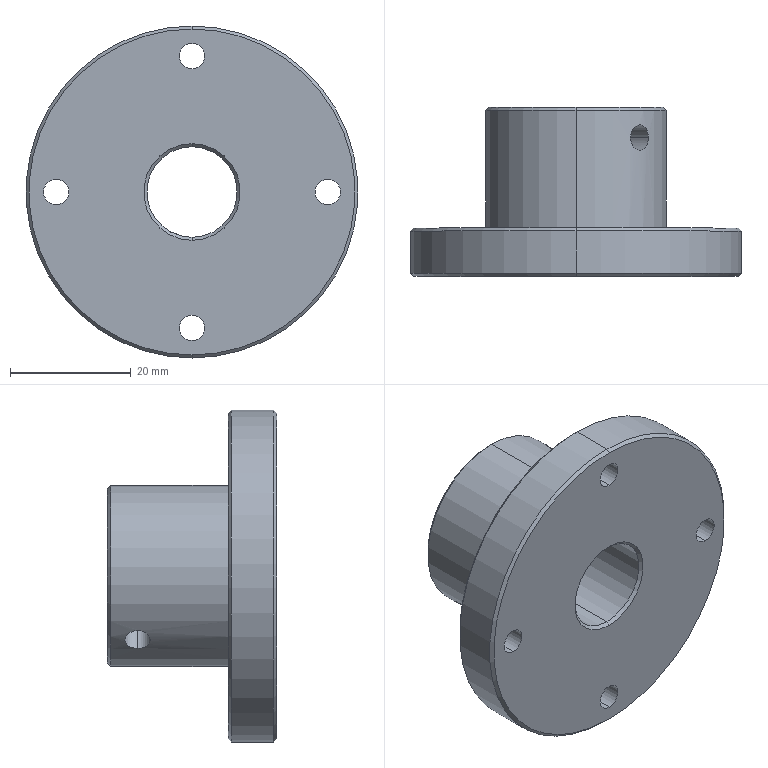Part | STEP file | 10000020598swp000-1 | 1 solid | 31 faces | box 55 x 28 x 55 mm | volume 27477 mm3 | cylinder 18 | cone 10 | plane 3 | commonest cylinder face diameters 4.2 x12 15 x2 30 x2 55 x2
STEP:
#1=CARTESIAN_POINT('',(-11.987,23.,-9.017));
#2=VERTEX_POINT('',#1);
#3=CARTESIAN_POINT('',(-9.017,23.,-11.987));
#4=VERTEX_POINT('',#3);
#5=CARTESIAN_POINT('',(-11.987,23.,-9.017));
#6=CARTESIAN_POINT('',(-11.987,22.726,-9.017));
#7=CARTESIAN_POINT('',(-11.954,22.449,-9.062));
#8=CARTESIAN_POINT('',(-11.857,22.07,-9.187));
#9=CARTESIAN_POINT('',(-11.817,21.948,-9.239));
#10=CARTESIAN_POINT('',(-11.721,21.719,-9.36));
#11=CARTESIAN_POINT('',(-11.667,21.613,-9.429));
#12=CARTESIAN_POINT('',(-11.544,21.419,-9.579));
#13=CARTESIAN_POINT('',(-11.474,21.331,-9.662));
#14=CARTESIAN_POINT('',(-11.326,21.178,-9.836));
#15=CARTESIAN_POINT('',(-11.246,21.114,-9.927));
#16=CARTESIAN_POINT('',(-11.076,21.008,-10.116));
#17=CARTESIAN_POINT('',(-10.986,20.967,-10.214));
#18=CARTESIAN_POINT('',(-10.801,20.914,-10.409));
#19=CARTESIAN_POINT('',(-10.706,20.9,-10.507));
#20=CARTESIAN_POINT('',(-10.509,20.9,-10.704));
#21=CARTESIAN_POINT('',(-10.412,20.913,-10.799));
#22=CARTESIAN_POINT('',(-10.216,20.967,-10.984));
#23=CARTESIAN_POINT('',(-10.118,21.007,-11.074));
#24=CARTESIAN_POINT('',(-9.929,21.112,-11.244));
#25=CARTESIAN_POINT('',(-9.838,21.177,-11.324));
#26=CARTESIAN_POINT('',(-9.664,21.329,-11.473));
#27=CARTESIAN_POINT('',(-9.581,21.417,-11.542));
#28=CARTESIAN_POINT('',(-9.355,21.707,-11.727));
#29=CARTESIAN_POINT('',(-9.23,21.941,-11.824));
#30=CARTESIAN_POINT('',(-9.063,22.446,-11.953));
#31=CARTESIAN_POINT('',(-9.017,22.722,-11.987));
#32=CARTESIAN_POINT('',(-9.017,23.,-11.987));
#33=B_SPLINE_CURVE_WITH_KNOTS('',3,(#5,#6,#7,#8,#9,#10,#11,#12,#13,#14,#15,#16,#17,#18,#19,#20,#21,#22,#23,#24,#25,#26,#27,#28,#29,#30,#31,#32),.UNSPECIFIED.,.F.,.F.,(4,2,2,2,2,2,2,2,2,2,2,2,2,4),(0.006574,0.007395,0.007806,0.008217,0.008627,0.009038,0.009449,0.00986,0.01027,0.01068,0.01109,0.0115,0.01232,0.01315),.UNSPECIFIED.);
#34=EDGE_CURVE('',#2,#4,#33,.T.);
#35=ORIENTED_EDGE('',*,*,#34,.F.);
#36=CARTESIAN_POINT('',(-6.576,23.,-3.606));
#37=VERTEX_POINT('',#36);
#38=CARTESIAN_POINT('',(-1.485,23.,1.485));
#39=DIRECTION('',(0.7071,0.,0.7071));
#40=VECTOR('',#39,1000.);
#41=LINE('',#38,#40);
#42=EDGE_CURVE('',#2,#37,#41,.T.);
#43=ORIENTED_EDGE('',*,*,#42,.T.);
#44=CARTESIAN_POINT('',(-3.606,23.,-6.576));
#45=VERTEX_POINT('',#44);
#46=CARTESIAN_POINT('',(-3.606,23.,-6.576));
#47=CARTESIAN_POINT('',(-3.606,22.86,-6.576));
#48=CARTESIAN_POINT('',(-3.619,22.723,-6.569));
#49=CARTESIAN_POINT('',(-3.668,22.454,-6.542));
#50=CARTESIAN_POINT('',(-3.705,22.32,-6.521));
#51=CARTESIAN_POINT('',(-3.799,22.066,-6.467));
#52=CARTESIAN_POINT('',(-3.857,21.946,-6.433));
#53=CARTESIAN_POINT('',(-3.99,21.718,-6.351));
#54=CARTESIAN_POINT('',(-4.067,21.611,-6.303));
#55=CARTESIAN_POINT('',(-4.312,21.322,-6.139));
#56=CARTESIAN_POINT('',(-4.505,21.166,-6.002));
#57=CARTESIAN_POINT('',(-4.801,21.008,-5.763));
#58=CARTESIAN_POINT('',(-4.903,20.968,-5.677));
#59=CARTESIAN_POINT('',(-5.106,20.914,-5.495));
#60=CARTESIAN_POINT('',(-5.205,20.9,-5.401));
#61=CARTESIAN_POINT('',(-5.4,20.9,-5.207));
#62=CARTESIAN_POINT('',(-5.496,20.914,-5.105));
#63=CARTESIAN_POINT('',(-5.677,20.968,-4.903));
#64=CARTESIAN_POINT('',(-5.762,21.008,-4.803));
#65=CARTESIAN_POINT('',(-6.003,21.167,-4.503));
#66=CARTESIAN_POINT('',(-6.139,21.321,-4.313));
#67=CARTESIAN_POINT('',(-6.303,21.613,-4.065));
#68=CARTESIAN_POINT('',(-6.351,21.718,-3.99));
#69=CARTESIAN_POINT('',(-6.432,21.945,-3.857));
#70=CARTESIAN_POINT('',(-6.467,22.068,-3.799));
#71=CARTESIAN_POINT('',(-6.522,22.321,-3.704));
#72=CARTESIAN_POINT('',(-6.542,22.452,-3.668));
#73=CARTESIAN_POINT('',(-6.569,22.723,-3.619));
#74=CARTESIAN_POINT('',(-6.576,22.863,-3.606));
#75=CARTESIAN_POINT('',(-6.576,23.,-3.606));
#76=B_SPLINE_CURVE_WITH_KNOTS('',3,(#46,#47,#48,#49,#50,#51,#52,#53,#54,#55,#56,#57,#58,#59,#60,#61,#62,#63,#64,#65,#66,#67,#68,#69,#70,#71,#72,#73,#74,#75),.UNSPECIFIED.,.F.,.F.,(4,2,2,2,2,2,2,2,2,2,2,2,2,2,4),(0.,0.0004124,0.0008248,0.001237,0.00165,0.002474,0.002887,0.003299,0.003712,0.004124,0.004949,0.005361,0.005774,0.006186,0.006599),.UNSPECIFIED.);
#77=EDGE_CURVE('',#45,#37,#76,.T.);
#78=ORIENTED_EDGE('',*,*,#77,.F.);
#79=CARTESIAN_POINT('',(1.485,23.,-1.485));
#80=DIRECTION('',(0.7071,0.,0.7071));
#81=VECTOR('',#80,1000.);
#82=LINE('',#79,#81);
#83=EDGE_CURVE('',#4,#45,#82,.T.);
#84=ORIENTED_EDGE('',*,*,#83,.F.);
#85=EDGE_LOOP('',(#35,#43,#78,#84));
#86=FACE_OUTER_BOUND('',#85,.T.);
#87=CARTESIAN_POINT('',(0.,23.,0.));
#88=DIRECTION('',(0.7071,0.,0.7071));
#89=DIRECTION('',(0.7071,0.,-0.7071));
#90=AXIS2_PLACEMENT_3D('',#87,#88,#89);
#91=CYLINDRICAL_SURFACE('',#90,2.1);
#92=ADVANCED_FACE('',(#86),#91,.F.);
#93=CARTESIAN_POINT('',(11.987,23.,9.017));
#94=VERTEX_POINT('',#93);
#95=CARTESIAN_POINT('',(9.017,23.,11.987));
#96=VERTEX_POINT('',#95);
#97=CARTESIAN_POINT('',(11.987,23.,9.017));
#98=CARTESIAN_POINT('',(11.987,22.726,9.017));
#99=CARTESIAN_POINT('',(11.954,22.449,9.062));
#100=CARTESIAN_POINT('',(11.857,22.07,9.187));
#101=CARTESIAN_POINT('',(11.817,21.948,9.239));
#102=CARTESIAN_POINT('',(11.721,21.719,9.36));
#103=CARTESIAN_POINT('',(11.667,21.613,9.429));
#104=CARTESIAN_POINT('',(11.544,21.419,9.579));
#105=CARTESIAN_POINT('',(11.474,21.331,9.662));
#106=CARTESIAN_POINT('',(11.326,21.178,9.836));
#107=CARTESIAN_POINT('',(11.246,21.114,9.927));
#108=CARTESIAN_POINT('',(11.076,21.008,10.116));
#109=CARTESIAN_POINT('',(10.986,20.967,10.214));
#110=CARTESIAN_POINT('',(10.801,20.914,10.409));
#111=CARTESIAN_POINT('',(10.706,20.9,10.507));
#112=CARTESIAN_POINT('',(10.509,20.9,10.704));
#113=CARTESIAN_POINT('',(10.412,20.913,10.799));
#114=CARTESIAN_POINT('',(10.216,20.967,10.984));
#115=CARTESIAN_POINT('',(10.118,21.007,11.074));
#116=CARTESIAN_POINT('',(9.929,21.112,11.244));
#117=CARTESIAN_POINT('',(9.838,21.177,11.324));
#118=CARTESIAN_POINT('',(9.664,21.329,11.473));
#119=CARTESIAN_POINT('',(9.581,21.417,11.542));
#120=CARTESIAN_POINT('',(9.355,21.707,11.727));
#121=CARTESIAN_POINT('',(9.23,21.941,11.824));
#122=CARTESIAN_POINT('',(9.063,22.446,11.953));
#123=CARTESIAN_POINT('',(9.017,22.722,11.987));
#124=CARTESIAN_POINT('',(9.017,23.,11.987));
#125=B_SPLINE_CURVE_WITH_KNOTS('',3,(#97,#98,#99,#100,#101,#102,#103,#104,#105,#106,#107,#108,#109,#110,#111,#112,#113,#114,#115,#116,#117,#118,#119,#120,#121,#122,#123,#124),.UNSPECIFIED.,.F.,.F.,(4,2,2,2,2,2,2,2,2,2,2,2,2,4),(0.006574,0.007395,0.007806,0.008217,0.008627,0.009038,0.009449,0.00986,0.01027,0.01068,0.01109,0.0115,0.01232,0.01315),.UNSPECIFIED.);
#126=EDGE_CURVE('',#94,#96,#125,.T.);
#127=ORIENTED_EDGE('',*,*,#126,.F.);
#128=CARTESIAN_POINT('',(6.576,23.,3.606));
#129=VERTEX_POINT('',#128);
#130=CARTESIAN_POINT('',(1.485,23.,-1.485));
#131=DIRECTION('',(-0.7071,0.,-0.7071));
#132=VECTOR('',#131,1000.);
#133=LINE('',#130,#132);
#134=EDGE_CURVE('',#94,#129,#133,.T.);
#135=ORIENTED_EDGE('',*,*,#134,.T.);
#136=CARTESIAN_POINT('',(3.606,23.,6.576));
#137=VERTEX_POINT('',#136);
#138=CARTESIAN_POINT('',(3.606,23.,6.576));
#139=CARTESIAN_POINT('',(3.606,22.86,6.576));
#140=CARTESIAN_POINT('',(3.619,22.723,6.569));
#141=CARTESIAN_POINT('',(3.668,22.454,6.542));
#142=CARTESIAN_POINT('',(3.705,22.32,6.521));
#143=CARTESIAN_POINT('',(3.799,22.066,6.467));
#144=CARTESIAN_POINT('',(3.857,21.946,6.433));
#145=CARTESIAN_POINT('',(3.99,21.718,6.351));
#146=CARTESIAN_POINT('',(4.067,21.611,6.303));
#147=CARTESIAN_POINT('',(4.312,21.322,6.139));
#148=CARTESIAN_POINT('',(4.505,21.166,6.002));
#149=CARTESIAN_POINT('',(4.801,21.008,5.763));
#150=CARTESIAN_POINT('',(4.903,20.968,5.677));
#151=CARTESIAN_POINT('',(5.106,20.914,5.495));
#152=CARTESIAN_POINT('',(5.205,20.9,5.401));
#153=CARTESIAN_POINT('',(5.4,20.9,5.207));
#154=CARTESIAN_POINT('',(5.496,20.914,5.105));
#155=CARTESIAN_POINT('',(5.677,20.968,4.903));
#156=CARTESIAN_POINT('',(5.762,21.008,4.803));
#157=CARTESIAN_POINT('',(6.003,21.167,4.503));
#158=CARTESIAN_POINT('',(6.139,21.321,4.313));
#159=CARTESIAN_POINT('',(6.303,21.613,4.065));
#160=CARTESIAN_POINT('',(6.351,21.718,3.99));
#161=CARTESIAN_POINT('',(6.432,21.945,3.857));
#162=CARTESIAN_POINT('',(6.467,22.068,3.799));
#163=CARTESIAN_POINT('',(6.522,22.321,3.704));
#164=CARTESIAN_POINT('',(6.542,22.452,3.668));
#165=CARTESIAN_POINT('',(6.569,22.723,3.619));
#166=CARTESIAN_POINT('',(6.576,22.863,3.606));
#167=CARTESIAN_POINT('',(6.576,23.,3.606));
#168=B_SPLINE_CURVE_WITH_KNOTS('',3,(#138,#139,#140,#141,#142,#143,#144,#145,#146,#147,#148,#149,#150,#151,#152,#153,#154,#155,#156,#157,#158,#159,#160,#161,#162,#163,#164,#165,#166,#167),.UNSPECIFIED.,.F.,.F.,(4,2,2,2,2,2,2,2,2,2,2,2,2,2,4),(0.,0.0004124,0.0008248,0.001237,0.00165,0.002474,0.002887,0.003299,0.003712,0.004124,0.004949,0.005361,0.005774,0.006186,0.006599),.UNSPECIFIED.);
#169=EDGE_CURVE('',#137,#129,#168,.T.);
#170=ORIENTED_EDGE('',*,*,#169,.F.);
#171=CARTESIAN_POINT('',(-1.485,23.,1.485));
#172=DIRECTION('',(-0.7071,0.,-0.7071));
#173=VECTOR('',#172,1000.);
#174=LINE('',#171,#173);
#175=EDGE_CURVE('',#96,#137,#174,.T.);
#176=ORIENTED_EDGE('',*,*,#175,.F.);
#177=EDGE_LOOP('',(#127,#135,#170,#176));
#178=FACE_OUTER_BOUND('',#177,.T.);
#179=CARTESIAN_POINT('',(0.,23.,0.));
#180=DIRECTION('',(-0.7071,0.,-0.7071));
#181=DIRECTION('',(-0.7071,0.,0.7071));
#182=AXIS2_PLACEMENT_3D('',#179,#180,#181);
#183=CYLINDRICAL_SURFACE('',#182,2.1);
#184=ADVANCED_FACE('',(#178),#183,.F.);
#185=CARTESIAN_POINT('',(0.,28.,14.5));
#186=VERTEX_POINT('',#185);
#187=CARTESIAN_POINT('',(0.,28.,-14.5));
#188=VERTEX_POINT('',#187);
#189=CARTESIAN_POINT('',(0.,28.,0.));
#190=DIRECTION('',(0.,1.,0.));
#191=DIRECTION('',(0.,0.,1.));
#192=AXIS2_PLACEMENT_3D('',#189,#190,#191);
#193=CIRCLE('',#192,14.5);
#194=EDGE_CURVE('',#186,#188,#193,.T.);
#195=ORIENTED_EDGE('',*,*,#194,.F.);
#196=CARTESIAN_POINT('',(0.,27.5,15.));
#197=VERTEX_POINT('',#196);
#198=CARTESIAN_POINT('',(0.,28.,14.5));
#199=DIRECTION('',(0.,-0.7071,0.7071));
#200=VECTOR('',#199,1000.);
#201=LINE('',#198,#200);
#202=EDGE_CURVE('',#186,#197,#201,.T.);
#203=ORIENTED_EDGE('',*,*,#202,.T.);
#204=CARTESIAN_POINT('',(0.,27.5,-15.));
#205=VERTEX_POINT('',#204);
#206=CARTESIAN_POINT('',(0.,27.5,0.));
#207=DIRECTION('',(0.,-1.,0.));
#208=DIRECTION('',(0.,0.,1.));
#209=AXIS2_PLACEMENT_3D('',#206,#207,#208);
#210=CIRCLE('',#209,15.);
#211=EDGE_CURVE('',#205,#197,#210,.T.);
#212=ORIENTED_EDGE('',*,*,#211,.F.);
#213=CARTESIAN_POINT('',(0.,28.,-14.5));
#214=DIRECTION('',(0.,-0.7071,-0.7071));
#215=VECTOR('',#214,1000.);
#216=LINE('',#213,#215);
#217=EDGE_CURVE('',#188,#205,#216,.T.);
#218=ORIENTED_EDGE('',*,*,#217,.F.);
#219=EDGE_LOOP('',(#195,#203,#212,#218));
#220=FACE_OUTER_BOUND('',#219,.T.);
#221=CARTESIAN_POINT('',(0.,28.,0.));
#222=DIRECTION('',(0.,-1.,0.));
#223=DIRECTION('',(0.,0.,-1.));
#224=AXIS2_PLACEMENT_3D('',#221,#222,#223);
#225=CONICAL_SURFACE('',#224,14.5,0.7854);
#226=ADVANCED_FACE('',(#220),#225,.T.);
#227=CARTESIAN_POINT('',(0.,27.5,-7.5));
#228=VERTEX_POINT('',#227);
#229=CARTESIAN_POINT('',(0.,27.5,7.5));
#230=VERTEX_POINT('',#229);
#231=CARTESIAN_POINT('',(0.,27.5,0.));
#232=DIRECTION('',(0.,1.,0.));
#233=DIRECTION('',(0.,0.,1.));
#234=AXIS2_PLACEMENT_3D('',#231,#232,#233);
#235=CIRCLE('',#234,7.5);
#236=EDGE_CURVE('',#228,#230,#235,.T.);
#237=ORIENTED_EDGE('',*,*,#236,.F.);
#238=CARTESIAN_POINT('',(0.,28.,-8.));
#239=VERTEX_POINT('',#238);
#240=CARTESIAN_POINT('',(0.,27.5,-7.5));
#241=DIRECTION('',(0.,0.7071,-0.7071));
#242=VECTOR('',#241,1000.);
#243=LINE('',#240,#242);
#244=EDGE_CURVE('',#228,#239,#243,.T.);
#245=ORIENTED_EDGE('',*,*,#244,.T.);
#246=CARTESIAN_POINT('',(0.,28.,8.));
#247=VERTEX_POINT('',#246);
#248=CARTESIAN_POINT('',(0.,28.,0.));
#249=DIRECTION('',(0.,-1.,0.));
#250=DIRECTION('',(0.,0.,1.));
#251=AXIS2_PLACEMENT_3D('',#248,#249,#250);
#252=CIRCLE('',#251,8.);
#253=EDGE_CURVE('',#247,#239,#252,.T.);
#254=ORIENTED_EDGE('',*,*,#253,.F.);
#255=CARTESIAN_POINT('',(0.,27.5,7.5));
#256=DIRECTION('',(0.,0.7071,0.7071));
#257=VECTOR('',#256,1000.);
#258=LINE('',#255,#257);
#259=EDGE_CURVE('',#230,#247,#258,.T.);
#260=ORIENTED_EDGE('',*,*,#259,.F.);
#261=EDGE_LOOP('',(#237,#245,#254,#260));
#262=FACE_OUTER_BOUND('',#261,.T.);
#263=CARTESIAN_POINT('',(0.,27.5,0.));
#264=DIRECTION('',(0.,1.,0.));
#265=DIRECTION('',(0.,0.,1.));
#266=AXIS2_PLACEMENT_3D('',#263,#264,#265);
#267=CONICAL_SURFACE('',#266,7.5,0.7854);
#268=ADVANCED_FACE('',(#262),#267,.F.);
#269=CARTESIAN_POINT('',(0.,0.5,7.5));
#270=VERTEX_POINT('',#269);
#271=CARTESIAN_POINT('',(0.,0.5,-7.5));
#272=VERTEX_POINT('',#271);
#273=CARTESIAN_POINT('',(0.,0.5,0.));
#274=DIRECTION('',(0.,-1.,0.));
#275=DIRECTION('',(0.,0.,1.));
#276=AXIS2_PLACEMENT_3D('',#273,#274,#275);
#277=CIRCLE('',#276,7.5);
#278=EDGE_CURVE('',#270,#272,#277,.T.);
#279=ORIENTED_EDGE('',*,*,#278,.F.);
#280=CARTESIAN_POINT('',(0.,0.,8.));
#281=VERTEX_POINT('',#280);
#282=CARTESIAN_POINT('',(0.,0.,8.));
#283=DIRECTION('',(0.,-0.7071,0.7071));
#284=VECTOR('',#283,1000.);
#285=LINE('',#282,#284);
#286=EDGE_CURVE('',#270,#281,#285,.T.);
#287=ORIENTED_EDGE('',*,*,#286,.T.);
#288=CARTESIAN_POINT('',(0.,0.,-8.));
#289=VERTEX_POINT('',#288);
#290=CARTESIAN_POINT('',(0.,0.,0.));
#291=DIRECTION('',(0.,1.,0.));
#292=DIRECTION('',(0.,0.,1.));
#293=AXIS2_PLACEMENT_3D('',#290,#291,#292);
#294=CIRCLE('',#293,8.);
#295=EDGE_CURVE('',#289,#281,#294,.T.);
#296=ORIENTED_EDGE('',*,*,#295,.F.);
#297=CARTESIAN_POINT('',(0.,0.,-8.));
#298=DIRECTION('',(0.,-0.7071,-0.7071));
#299=VECTOR('',#298,1000.);
#300=LINE('',#297,#299);
#301=EDGE_CURVE('',#272,#289,#300,.T.);
#302=ORIENTED_EDGE('',*,*,#301,.F.);
#303=EDGE_LOOP('',(#279,#287,#296,#302));
#304=FACE_OUTER_BOUND('',#303,.T.);
#305=CARTESIAN_POINT('',(0.,0.,0.));
#306=DIRECTION('',(0.,-1.,0.));
#307=DIRECTION('',(0.,0.,-1.));
#308=AXIS2_PLACEMENT_3D('',#305,#306,#307);
#309=CONICAL_SURFACE('',#308,8.,0.7854);
#310=ADVANCED_FACE('',(#304),#309,.F.);
#311=CARTESIAN_POINT('',(0.,8.,-24.6));
#312=VERTEX_POINT('',#311);
#313=CARTESIAN_POINT('',(0.,8.,-20.4));
#314=VERTEX_POINT('',#313);
#315=CARTESIAN_POINT('',(0.,8.,-22.5));
#316=DIRECTION('',(0.,1.,0.));
#317=DIRECTION('',(0.,0.,1.));
#318=AXIS2_PLACEMENT_3D('',#315,#316,#317);
#319=CIRCLE('',#318,2.1);
#320=EDGE_CURVE('',#312,#314,#319,.T.);
#321=ORIENTED_EDGE('',*,*,#320,.T.);
#322=CARTESIAN_POINT('',(0.,0.,-20.4));
#323=VERTEX_POINT('',#322);
#324=CARTESIAN_POINT('',(0.,0.,-20.4));
#325=DIRECTION('',(0.,-1.,0.));
#326=VECTOR('',#325,1000.);
#327=LINE('',#324,#326);
#328=EDGE_CURVE('',#314,#323,#327,.T.);
#329=ORIENTED_EDGE('',*,*,#328,.T.);
#330=CARTESIAN_POINT('',(0.,0.,-24.6));
#331=VERTEX_POINT('',#330);
#332=CARTESIAN_POINT('',(0.,0.,-22.5));
#333=DIRECTION('',(0.,-1.,0.));
#334=DIRECTION('',(0.,0.,-1.));
#335=AXIS2_PLACEMENT_3D('',#332,#333,#334);
#336=CIRCLE('',#335,2.1);
#337=EDGE_CURVE('',#323,#331,#336,.T.);
#338=ORIENTED_EDGE('',*,*,#337,.T.);
#339=CARTESIAN_POINT('',(0.,0.,-24.6));
#340=DIRECTION('',(0.,-1.,0.));
#341=VECTOR('',#340,1000.);
#342=LINE('',#339,#341);
#343=EDGE_CURVE('',#312,#331,#342,.T.);
#344=ORIENTED_EDGE('',*,*,#343,.F.);
#345=EDGE_LOOP('',(#321,#329,#338,#344));
#346=FACE_OUTER_BOUND('',#345,.T.);
#347=CARTESIAN_POINT('',(0.,0.,-22.5));
#348=DIRECTION('',(0.,-1.,0.));
#349=DIRECTION('',(0.,0.,-1.));
#350=AXIS2_PLACEMENT_3D('',#347,#348,#349);
#351=CYLINDRICAL_SURFACE('',#350,2.1);
#352=ADVANCED_FACE('',(#346),#351,.F.);
#353=CARTESIAN_POINT('',(-22.5,8.,-2.1));
#354=VERTEX_POINT('',#353);
#355=CARTESIAN_POINT('',(-22.5,8.,2.1));
#356=VERTEX_POINT('',#355);
#357=CARTESIAN_POINT('',(-22.5,8.,0.));
#358=DIRECTION('',(0.,1.,0.));
#359=DIRECTION('',(0.,0.,1.));
#360=AXIS2_PLACEMENT_3D('',#357,#358,#359);
#361=CIRCLE('',#360,2.1);
#362=EDGE_CURVE('',#354,#356,#361,.T.);
#363=ORIENTED_EDGE('',*,*,#362,.T.);
#364=CARTESIAN_POINT('',(-22.5,0.,2.1));
#365=VERTEX_POINT('',#364);
#366=CARTESIAN_POINT('',(-22.5,0.,2.1));
#367=DIRECTION('',(0.,-1.,0.));
#368=VECTOR('',#367,1000.);
#369=LINE('',#366,#368);
#370=EDGE_CURVE('',#356,#365,#369,.T.);
#371=ORIENTED_EDGE('',*,*,#370,.T.);
#372=CARTESIAN_POINT('',(-22.5,0.,-2.1));
#373=VERTEX_POINT('',#372);
#374=CARTESIAN_POINT('',(-22.5,0.,0.));
#375=DIRECTION('',(0.,-1.,0.));
#376=DIRECTION('',(0.,0.,-1.));
#377=AXIS2_PLACEMENT_3D('',#374,#375,#376);
#378=CIRCLE('',#377,2.1);
#379=EDGE_CURVE('',#365,#373,#378,.T.);
#380=ORIENTED_EDGE('',*,*,#379,.T.);
#381=CARTESIAN_POINT('',(-22.5,0.,-2.1));
#382=DIRECTION('',(0.,-1.,0.));
#383=VECTOR('',#382,1000.);
#384=LINE('',#381,#383);
#385=EDGE_CURVE('',#354,#373,#384,.T.);
#386=ORIENTED_EDGE('',*,*,#385,.F.);
#387=EDGE_LOOP('',(#363,#371,#380,#386));
#388=FACE_OUTER_BOUND('',#387,.T.);
#389=CARTESIAN_POINT('',(-22.5,0.,0.));
#390=DIRECTION('',(0.,-1.,0.));
#391=DIRECTION('',(0.,0.,-1.));
#392=AXIS2_PLACEMENT_3D('',#389,#390,#391);
#393=CYLINDRICAL_SURFACE('',#392,2.1);
#394=ADVANCED_FACE('',(#388),#393,.F.);
#395=CARTESIAN_POINT('',(0.,8.,20.4));
#396=VERTEX_POINT('',#395);
#397=CARTESIAN_POINT('',(0.,8.,24.6));
#398=VERTEX_POINT('',#397);
#399=CARTESIAN_POINT('',(0.,8.,22.5));
#400=DIRECTION('',(0.,1.,0.));
#401=DIRECTION('',(0.,0.,1.));
#402=AXIS2_PLACEMENT_3D('',#399,#400,#401);
#403=CIRCLE('',#402,2.1);
#404=EDGE_CURVE('',#396,#398,#403,.T.);
#405=ORIENTED_EDGE('',*,*,#404,.T.);
#406=CARTESIAN_POINT('',(0.,0.,24.6));
#407=VERTEX_POINT('',#406);
#408=CARTESIAN_POINT('',(0.,0.,24.6));
#409=DIRECTION('',(0.,-1.,0.));
#410=VECTOR('',#409,1000.);
#411=LINE('',#408,#410);
#412=EDGE_CURVE('',#398,#407,#411,.T.);
#413=ORIENTED_EDGE('',*,*,#412,.T.);
#414=CARTESIAN_POINT('',(0.,0.,20.4));
#415=VERTEX_POINT('',#414);
#416=CARTESIAN_POINT('',(0.,0.,22.5));
#417=DIRECTION('',(0.,-1.,0.));
#418=DIRECTION('',(0.,0.,-1.));
#419=AXIS2_PLACEMENT_3D('',#416,#417,#418);
#420=CIRCLE('',#419,2.1);
#421=EDGE_CURVE('',#407,#415,#420,.T.);
#422=ORIENTED_EDGE('',*,*,#421,.T.);
#423=CARTESIAN_POINT('',(0.,0.,20.4));
#424=DIRECTION('',(0.,-1.,0.));
#425=VECTOR('',#424,1000.);
#426=LINE('',#423,#425);
#427=EDGE_CURVE('',#396,#415,#426,.T.);
#428=ORIENTED_EDGE('',*,*,#427,.F.);
#429=EDGE_LOOP('',(#405,#413,#422,#428));
#430=FACE_OUTER_BOUND('',#429,.T.);
#431=CARTESIAN_POINT('',(0.,0.,22.5));
#432=DIRECTION('',(0.,-1.,0.));
#433=DIRECTION('',(0.,0.,-1.));
#434=AXIS2_PLACEMENT_3D('',#431,#432,#433);
#435=CYLINDRICAL_SURFACE('',#434,2.1);
#436=ADVANCED_FACE('',(#430),#435,.F.);
#437=CARTESIAN_POINT('',(22.5,8.,-2.1));
#438=VERTEX_POINT('',#437);
#439=CARTESIAN_POINT('',(22.5,8.,2.1));
#440=VERTEX_POINT('',#439);
#441=CARTESIAN_POINT('',(22.5,8.,0.));
#442=DIRECTION('',(0.,1.,0.));
#443=DIRECTION('',(0.,0.,1.));
#444=AXIS2_PLACEMENT_3D('',#441,#442,#443);
#445=CIRCLE('',#444,2.1);
#446=EDGE_CURVE('',#438,#440,#445,.T.);
#447=ORIENTED_EDGE('',*,*,#446,.T.);
#448=CARTESIAN_POINT('',(22.5,0.,2.1));
#449=VERTEX_POINT('',#448);
#450=CARTESIAN_POINT('',(22.5,0.,2.1));
#451=DIRECTION('',(0.,-1.,0.));
#452=VECTOR('',#451,1000.);
#453=LINE('',#450,#452);
#454=EDGE_CURVE('',#440,#449,#453,.T.);
#455=ORIENTED_EDGE('',*,*,#454,.T.);
#456=CARTESIAN_POINT('',(22.5,0.,-2.1));
#457=VERTEX_POINT('',#456);
#458=CARTESIAN_POINT('',(22.5,0.,0.));
#459=DIRECTION('',(0.,-1.,0.));
#460=DIRECTION('',(0.,0.,-1.));
#461=AXIS2_PLACEMENT_3D('',#458,#459,#460);
#462=CIRCLE('',#461,2.1);
#463=EDGE_CURVE('',#449,#457,#462,.T.);
#464=ORIENTED_EDGE('',*,*,#463,.T.);
#465=CARTESIAN_POINT('',(22.5,0.,-2.1));
#466=DIRECTION('',(0.,-1.,0.));
#467=VECTOR('',#466,1000.);
#468=LINE('',#465,#467);
#469=EDGE_CURVE('',#438,#457,#468,.T.);
#470=ORIENTED_EDGE('',*,*,#469,.F.);
#471=EDGE_LOOP('',(#447,#455,#464,#470));
#472=FACE_OUTER_BOUND('',#471,.T.);
#473=CARTESIAN_POINT('',(22.5,0.,0.));
#474=DIRECTION('',(0.,-1.,0.));
#475=DIRECTION('',(0.,0.,-1.));
#476=AXIS2_PLACEMENT_3D('',#473,#474,#475);
#477=CYLINDRICAL_SURFACE('',#476,2.1);
#478=ADVANCED_FACE('',(#472),#477,.F.);
#479=ORIENTED_EDGE('',*,*,#77,.T.);
#480=CARTESIAN_POINT('',(-6.576,23.,-3.606));
#481=CARTESIAN_POINT('',(-6.576,23.275,-3.606));
#482=CARTESIAN_POINT('',(-6.549,23.552,-3.657));
#483=CARTESIAN_POINT('',(-6.467,23.932,-3.799));
#484=CARTESIAN_POINT('',(-6.433,24.055,-3.857));
#485=CARTESIAN_POINT('',(-6.351,24.282,-3.991));
#486=CARTESIAN_POINT('',(-6.303,24.387,-4.066));
#487=CARTESIAN_POINT('',(-6.194,24.581,-4.23));
#488=CARTESIAN_POINT('',(-6.132,24.669,-4.32));
#489=CARTESIAN_POINT('',(-5.997,24.821,-4.505));
#490=CARTESIAN_POINT('',(-5.924,24.886,-4.602));
#491=CARTESIAN_POINT('',(-5.762,24.992,-4.803));
#492=CARTESIAN_POINT('',(-5.677,25.032,-4.903));
#493=CARTESIAN_POINT('',(-5.497,25.086,-5.104));
#494=CARTESIAN_POINT('',(-5.401,25.1,-5.205));
#495=CARTESIAN_POINT('',(-5.206,25.1,-5.401));
#496=CARTESIAN_POINT('',(-5.106,25.086,-5.495));
#497=CARTESIAN_POINT('',(-4.905,25.033,-5.676));
#498=CARTESIAN_POINT('',(-4.802,24.992,-5.762));
#499=CARTESIAN_POINT('',(-4.505,24.834,-6.002));
#500=CARTESIAN_POINT('',(-4.312,24.678,-6.139));
#501=CARTESIAN_POINT('',(-4.067,24.389,-6.302));
#502=CARTESIAN_POINT('',(-3.991,24.282,-6.351));
#503=CARTESIAN_POINT('',(-3.857,24.054,-6.433));
#504=CARTESIAN_POINT('',(-3.8,23.934,-6.467));
#505=CARTESIAN_POINT('',(-3.705,23.681,-6.521));
#506=CARTESIAN_POINT('',(-3.668,23.547,-6.542));
#507=CARTESIAN_POINT('',(-3.619,23.277,-6.569));
#508=CARTESIAN_POINT('',(-3.606,23.139,-6.576));
#509=CARTESIAN_POINT('',(-3.606,23.,-6.576));
#510=B_SPLINE_CURVE_WITH_KNOTS('',3,(#480,#481,#482,#483,#484,#485,#486,#487,#488,#489,#490,#491,#492,#493,#494,#495,#496,#497,#498,#499,#500,#501,#502,#503,#504,#505,#506,#507,#508,#509),.UNSPECIFIED.,.F.,.F.,(4,2,2,2,2,2,2,2,2,2,2,2,2,2,4),(0.006599,0.007423,0.007836,0.008248,0.00866,0.009072,0.009485,0.009897,0.01031,0.01072,0.01155,0.01196,0.01237,0.01278,0.0132),.UNSPECIFIED.);
#511=EDGE_CURVE('',#37,#45,#510,.T.);
#512=ORIENTED_EDGE('',*,*,#511,.T.);
#513=EDGE_LOOP('',(#479,#512));
#514=FACE_BOUND('',#513,.T.);
#515=ORIENTED_EDGE('',*,*,#278,.T.);
#516=CARTESIAN_POINT('',(0.,28.,-7.5));
#517=DIRECTION('',(0.,1.,0.));
#518=VECTOR('',#517,1000.);
#519=LINE('',#516,#518);
#520=EDGE_CURVE('',#272,#228,#519,.T.);
#521=ORIENTED_EDGE('',*,*,#520,.T.);
#522=ORIENTED_EDGE('',*,*,#236,.T.);
#523=CARTESIAN_POINT('',(0.,28.,7.5));
#524=DIRECTION('',(0.,1.,0.));
#525=VECTOR('',#524,1000.);
#526=LINE('',#523,#525);
#527=EDGE_CURVE('',#270,#230,#526,.T.);
#528=ORIENTED_EDGE('',*,*,#527,.F.);
#529=EDGE_LOOP('',(#515,#521,#522,#528));
#530=FACE_OUTER_BOUND('',#529,.T.);
#531=CARTESIAN_POINT('',(0.,28.,0.));
#532=DIRECTION('',(0.,1.,0.));
#533=DIRECTION('',(0.,0.,1.));
#534=AXIS2_PLACEMENT_3D('',#531,#532,#533);
#535=CYLINDRICAL_SURFACE('',#534,7.5);
#536=ADVANCED_FACE('',(#514,#530),#535,.F.);
#537=CARTESIAN_POINT('',(9.017,23.,11.987));
#538=CARTESIAN_POINT('',(9.017,23.139,11.987));
#539=CARTESIAN_POINT('',(9.028,23.276,11.979));
#540=CARTESIAN_POINT('',(9.071,23.544,11.946));
#541=CARTESIAN_POINT('',(9.104,23.678,11.922));
#542=CARTESIAN_POINT('',(9.188,23.932,11.857));
#543=CARTESIAN_POINT('',(9.24,24.052,11.817));
#544=CARTESIAN_POINT('',(9.36,24.281,11.722));
#545=CARTESIAN_POINT('',(9.43,24.389,11.666));
#546=CARTESIAN_POINT('',(9.655,24.679,11.481));
#547=CARTESIAN_POINT('',(9.834,24.835,11.329));
#548=CARTESIAN_POINT('',(10.211,25.045,10.991));
#549=CARTESIAN_POINT('',(10.412,25.1,10.801));
#550=CARTESIAN_POINT('',(10.703,25.1,10.51));
#551=CARTESIAN_POINT('',(10.8,25.086,10.41));
#552=CARTESIAN_POINT('',(10.986,25.033,10.215));
#553=CARTESIAN_POINT('',(11.074,24.993,10.118));
#554=CARTESIAN_POINT('',(11.245,24.888,9.928));
#555=CARTESIAN_POINT('',(11.326,24.822,9.836));
#556=CARTESIAN_POINT('',(11.474,24.67,9.663));
#557=CARTESIAN_POINT('',(11.542,24.583,9.581));
#558=CARTESIAN_POINT('',(11.667,24.387,9.428));
#559=CARTESIAN_POINT('',(11.721,24.281,9.36));
#560=CARTESIAN_POINT('',(11.816,24.054,9.24));
#561=CARTESIAN_POINT('',(11.857,23.931,9.188));
#562=CARTESIAN_POINT('',(11.922,23.677,9.104));
#563=CARTESIAN_POINT('',(11.946,23.546,9.072));
#564=CARTESIAN_POINT('',(11.979,23.276,9.028));
#565=CARTESIAN_POINT('',(11.987,23.137,9.017));
#566=CARTESIAN_POINT('',(11.987,23.,9.017));
#567=B_SPLINE_CURVE_WITH_KNOTS('',3,(#537,#538,#539,#540,#541,#542,#543,#544,#545,#546,#547,#548,#549,#550,#551,#552,#553,#554,#555,#556,#557,#558,#559,#560,#561,#562,#563,#564,#565,#566),.UNSPECIFIED.,.F.,.F.,(4,2,2,2,2,2,2,2,2,2,2,2,2,2,4),(0.,0.0004109,0.0008217,0.001233,0.001643,0.002465,0.003287,0.003698,0.004109,0.004519,0.00493,0.005341,0.005752,0.006163,0.006574),.UNSPECIFIED.);
#568=EDGE_CURVE('',#96,#94,#567,.T.);
#569=ORIENTED_EDGE('',*,*,#568,.T.);
#570=ORIENTED_EDGE('',*,*,#126,.T.);
#571=EDGE_LOOP('',(#569,#570));
#572=FACE_BOUND('',#571,.T.);
#573=ORIENTED_EDGE('',*,*,#211,.T.);
#574=CARTESIAN_POINT('',(0.,8.,15.));
#575=VERTEX_POINT('',#574);
#576=CARTESIAN_POINT('',(0.,28.,15.));
#577=DIRECTION('',(0.,-1.,0.));
#578=VECTOR('',#577,1000.);
#579=LINE('',#576,#578);
#580=EDGE_CURVE('',#197,#575,#579,.T.);
#581=ORIENTED_EDGE('',*,*,#580,.T.);
#582=CARTESIAN_POINT('',(0.,8.,-15.));
#583=VERTEX_POINT('',#582);
#584=CARTESIAN_POINT('',(0.,8.,0.));
#585=DIRECTION('',(0.,1.,0.));
#586=DIRECTION('',(0.,0.,1.));
#587=AXIS2_PLACEMENT_3D('',#584,#585,#586);
#588=CIRCLE('',#587,15.);
#589=EDGE_CURVE('',#575,#583,#588,.T.);
#590=ORIENTED_EDGE('',*,*,#589,.T.);
#591=CARTESIAN_POINT('',(0.,28.,-15.));
#592=DIRECTION('',(0.,-1.,0.));
#593=VECTOR('',#592,1000.);
#594=LINE('',#591,#593);
#595=EDGE_CURVE('',#205,#583,#594,.T.);
#596=ORIENTED_EDGE('',*,*,#595,.F.);
#597=EDGE_LOOP('',(#573,#581,#590,#596));
#598=FACE_OUTER_BOUND('',#597,.T.);
#599=CARTESIAN_POINT('',(0.,28.,0.));
#600=DIRECTION('',(0.,-1.,0.));
#601=DIRECTION('',(0.,0.,-1.));
#602=AXIS2_PLACEMENT_3D('',#599,#600,#601);
#603=CYLINDRICAL_SURFACE('',#602,15.);
#604=ADVANCED_FACE('',(#572,#598),#603,.T.);
#605=CARTESIAN_POINT('',(0.,0.,-27.));
#606=VERTEX_POINT('',#605);
#607=CARTESIAN_POINT('',(0.,0.,27.));
#608=VERTEX_POINT('',#607);
#609=CARTESIAN_POINT('',(0.,0.,0.));
#610=DIRECTION('',(0.,-1.,0.));
#611=DIRECTION('',(0.,0.,1.));
#612=AXIS2_PLACEMENT_3D('',#609,#610,#611);
#613=CIRCLE('',#612,27.);
#614=EDGE_CURVE('',#606,#608,#613,.T.);
#615=ORIENTED_EDGE('',*,*,#614,.F.);
#616=CARTESIAN_POINT('',(0.,0.5,-27.5));
#617=VERTEX_POINT('',#616);
#618=CARTESIAN_POINT('',(0.,0.5,-27.5));
#619=DIRECTION('',(0.,0.7071,-0.7071));
#620=VECTOR('',#619,1000.);
#621=LINE('',#618,#620);
#622=EDGE_CURVE('',#606,#617,#621,.T.);
#623=ORIENTED_EDGE('',*,*,#622,.T.);
#624=CARTESIAN_POINT('',(0.,0.5,27.5));
#625=VERTEX_POINT('',#624);
#626=CARTESIAN_POINT('',(0.,0.5,0.));
#627=DIRECTION('',(0.,1.,0.));
#628=DIRECTION('',(0.,0.,1.));
#629=AXIS2_PLACEMENT_3D('',#626,#627,#628);
#630=CIRCLE('',#629,27.5);
#631=EDGE_CURVE('',#625,#617,#630,.T.);
#632=ORIENTED_EDGE('',*,*,#631,.F.);
#633=CARTESIAN_POINT('',(0.,0.5,27.5));
#634=DIRECTION('',(0.,0.7071,0.7071));
#635=VECTOR('',#634,1000.);
#636=LINE('',#633,#635);
#637=EDGE_CURVE('',#608,#625,#636,.T.);
#638=ORIENTED_EDGE('',*,*,#637,.F.);
#639=EDGE_LOOP('',(#615,#623,#632,#638));
#640=FACE_OUTER_BOUND('',#639,.T.);
#641=CARTESIAN_POINT('',(0.,0.5,0.));
#642=DIRECTION('',(0.,1.,0.));
#643=DIRECTION('',(0.,0.,1.));
#644=AXIS2_PLACEMENT_3D('',#641,#642,#643);
#645=CONICAL_SURFACE('',#644,27.5,0.7854);
#646=ADVANCED_FACE('',(#640),#645,.T.);
#647=CARTESIAN_POINT('',(0.,8.,27.));
#648=VERTEX_POINT('',#647);
#649=CARTESIAN_POINT('',(0.,8.,-27.));
#650=VERTEX_POINT('',#649);
#651=CARTESIAN_POINT('',(0.,8.,0.));
#652=DIRECTION('',(0.,1.,0.));
#653=DIRECTION('',(0.,0.,1.));
#654=AXIS2_PLACEMENT_3D('',#651,#652,#653);
#655=CIRCLE('',#654,27.);
#656=EDGE_CURVE('',#648,#650,#655,.T.);
#657=ORIENTED_EDGE('',*,*,#656,.F.);
#658=CARTESIAN_POINT('',(0.,7.5,27.5));
#659=VERTEX_POINT('',#658);
#660=CARTESIAN_POINT('',(0.,8.,27.));
#661=DIRECTION('',(0.,-0.7071,0.7071));
#662=VECTOR('',#661,1000.);
#663=LINE('',#660,#662);
#664=EDGE_CURVE('',#648,#659,#663,.T.);
#665=ORIENTED_EDGE('',*,*,#664,.T.);
#666=CARTESIAN_POINT('',(0.,7.5,-27.5));
#667=VERTEX_POINT('',#666);
#668=CARTESIAN_POINT('',(0.,7.5,0.));
#669=DIRECTION('',(0.,-1.,0.));
#670=DIRECTION('',(0.,0.,1.));
#671=AXIS2_PLACEMENT_3D('',#668,#669,#670);
#672=CIRCLE('',#671,27.5);
#673=EDGE_CURVE('',#667,#659,#672,.T.);
#674=ORIENTED_EDGE('',*,*,#673,.F.);
#675=CARTESIAN_POINT('',(0.,8.,-27.));
#676=DIRECTION('',(0.,-0.7071,-0.7071));
#677=VECTOR('',#676,1000.);
#678=LINE('',#675,#677);
#679=EDGE_CURVE('',#650,#667,#678,.T.);
#680=ORIENTED_EDGE('',*,*,#679,.F.);
#681=EDGE_LOOP('',(#657,#665,#674,#680));
#682=FACE_OUTER_BOUND('',#681,.T.);
#683=CARTESIAN_POINT('',(0.,8.,0.));
#684=DIRECTION('',(0.,-1.,0.));
#685=DIRECTION('',(0.,0.,-1.));
#686=AXIS2_PLACEMENT_3D('',#683,#684,#685);
#687=CONICAL_SURFACE('',#686,27.,0.7854);
#688=ADVANCED_FACE('',(#682),#687,.T.);
#689=ORIENTED_EDGE('',*,*,#673,.T.);
#690=CARTESIAN_POINT('',(0.,8.,27.5));
#691=DIRECTION('',(0.,-1.,0.));
#692=VECTOR('',#691,1000.);
#693=LINE('',#690,#692);
#694=EDGE_CURVE('',#659,#625,#693,.T.);
#695=ORIENTED_EDGE('',*,*,#694,.T.);
#696=ORIENTED_EDGE('',*,*,#631,.T.);
#697=CARTESIAN_POINT('',(0.,8.,-27.5));
#698=DIRECTION('',(0.,-1.,0.));
#699=VECTOR('',#698,1000.);
#700=LINE('',#697,#699);
#701=EDGE_CURVE('',#667,#617,#700,.T.);
#702=ORIENTED_EDGE('',*,*,#701,.F.);
#703=EDGE_LOOP('',(#689,#695,#696,#702));
#704=FACE_OUTER_BOUND('',#703,.T.);
#705=CARTESIAN_POINT('',(0.,8.,0.));
#706=DIRECTION('',(0.,-1.,0.));
#707=DIRECTION('',(0.,0.,-1.));
#708=AXIS2_PLACEMENT_3D('',#705,#706,#707);
#709=CYLINDRICAL_SURFACE('',#708,27.5);
#710=ADVANCED_FACE('',(#704),#709,.T.);
#711=ORIENTED_EDGE('',*,*,#694,.F.);
#712=CARTESIAN_POINT('',(0.,7.5,0.));
#713=DIRECTION('',(0.,-1.,0.));
#714=DIRECTION('',(0.,0.,1.));
#715=AXIS2_PLACEMENT_3D('',#712,#713,#714);
#716=CIRCLE('',#715,27.5);
#717=EDGE_CURVE('',#659,#667,#716,.T.);
#718=ORIENTED_EDGE('',*,*,#717,.T.);
#719=ORIENTED_EDGE('',*,*,#701,.T.);
#720=CARTESIAN_POINT('',(0.,0.5,0.));
#721=DIRECTION('',(0.,1.,0.));
#722=DIRECTION('',(0.,0.,1.));
#723=AXIS2_PLACEMENT_3D('',#720,#721,#722);
#724=CIRCLE('',#723,27.5);
#725=EDGE_CURVE('',#617,#625,#724,.T.);
#726=ORIENTED_EDGE('',*,*,#725,.T.);
#727=EDGE_LOOP('',(#711,#718,#719,#726));
#728=FACE_OUTER_BOUND('',#727,.T.);
#729=CARTESIAN_POINT('',(0.,8.,0.));
#730=DIRECTION('',(0.,-1.,0.));
#731=DIRECTION('',(0.,0.,-1.));
#732=AXIS2_PLACEMENT_3D('',#729,#730,#731);
#733=CYLINDRICAL_SURFACE('',#732,27.5);
#734=ADVANCED_FACE('',(#728),#733,.T.);
#735=ORIENTED_EDGE('',*,*,#320,.F.);
#736=CARTESIAN_POINT('',(0.,8.,-22.5));
#737=DIRECTION('',(0.,1.,0.));
#738=DIRECTION('',(0.,0.,1.));
#739=AXIS2_PLACEMENT_3D('',#736,#737,#738);
#740=CIRCLE('',#739,2.1);
#741=EDGE_CURVE('',#314,#312,#740,.T.);
#742=ORIENTED_EDGE('',*,*,#741,.F.);
#743=EDGE_LOOP('',(#735,#742));
#744=FACE_BOUND('',#743,.T.);
#745=ORIENTED_EDGE('',*,*,#362,.F.);
#746=CARTESIAN_POINT('',(-22.5,8.,0.));
#747=DIRECTION('',(0.,1.,0.));
#748=DIRECTION('',(0.,0.,1.));
#749=AXIS2_PLACEMENT_3D('',#746,#747,#748);
#750=CIRCLE('',#749,2.1);
#751=EDGE_CURVE('',#356,#354,#750,.T.);
#752=ORIENTED_EDGE('',*,*,#751,.F.);
#753=EDGE_LOOP('',(#745,#752));
#754=FACE_BOUND('',#753,.T.);
#755=ORIENTED_EDGE('',*,*,#404,.F.);
#756=CARTESIAN_POINT('',(0.,8.,22.5));
#757=DIRECTION('',(0.,1.,0.));
#758=DIRECTION('',(0.,0.,1.));
#759=AXIS2_PLACEMENT_3D('',#756,#757,#758);
#760=CIRCLE('',#759,2.1);
#761=EDGE_CURVE('',#398,#396,#760,.T.);
#762=ORIENTED_EDGE('',*,*,#761,.F.);
#763=EDGE_LOOP('',(#755,#762));
#764=FACE_BOUND('',#763,.T.);
#765=ORIENTED_EDGE('',*,*,#446,.F.);
#766=CARTESIAN_POINT('',(22.5,8.,0.));
#767=DIRECTION('',(0.,1.,0.));
#768=DIRECTION('',(0.,0.,1.));
#769=AXIS2_PLACEMENT_3D('',#766,#767,#768);
#770=CIRCLE('',#769,2.1);
#771=EDGE_CURVE('',#440,#438,#770,.T.);
#772=ORIENTED_EDGE('',*,*,#771,.F.);
#773=EDGE_LOOP('',(#765,#772));
#774=FACE_BOUND('',#773,.T.);
#775=CARTESIAN_POINT('',(0.,8.,0.));
#776=DIRECTION('',(0.,1.,0.));
#777=DIRECTION('',(0.,0.,1.));
#778=AXIS2_PLACEMENT_3D('',#775,#776,#777);
#779=CIRCLE('',#778,15.);
#780=EDGE_CURVE('',#583,#575,#779,.T.);
#781=ORIENTED_EDGE('',*,*,#780,.F.);
#782=ORIENTED_EDGE('',*,*,#589,.F.);
#783=EDGE_LOOP('',(#781,#782));
#784=FACE_BOUND('',#783,.T.);
#785=CARTESIAN_POINT('',(0.,8.,0.));
#786=DIRECTION('',(0.,1.,0.));
#787=DIRECTION('',(0.,0.,1.));
#788=AXIS2_PLACEMENT_3D('',#785,#786,#787);
#789=CIRCLE('',#788,27.);
#790=EDGE_CURVE('',#650,#648,#789,.T.);
#791=ORIENTED_EDGE('',*,*,#790,.T.);
#792=ORIENTED_EDGE('',*,*,#656,.T.);
#793=EDGE_LOOP('',(#791,#792));
#794=FACE_OUTER_BOUND('',#793,.T.);
#795=CARTESIAN_POINT('',(0.,8.,0.));
#796=DIRECTION('',(0.,1.,0.));
#797=DIRECTION('',(0.,0.,1.));
#798=AXIS2_PLACEMENT_3D('',#795,#796,#797);
#799=PLANE('',#798);
#800=ADVANCED_FACE('',(#744,#754,#764,#774,#784,#794),#799,.T.);
#801=ORIENTED_EDGE('',*,*,#295,.T.);
#802=CARTESIAN_POINT('',(0.,0.,0.));
#803=DIRECTION('',(0.,1.,0.));
#804=DIRECTION('',(0.,0.,1.));
#805=AXIS2_PLACEMENT_3D('',#802,#803,#804);
#806=CIRCLE('',#805,8.);
#807=EDGE_CURVE('',#281,#289,#806,.T.);
#808=ORIENTED_EDGE('',*,*,#807,.T.);
#809=EDGE_LOOP('',(#801,#808));
#810=FACE_BOUND('',#809,.T.);
#811=CARTESIAN_POINT('',(0.,0.,-22.5));
#812=DIRECTION('',(0.,-1.,0.));
#813=DIRECTION('',(0.,0.,-1.));
#814=AXIS2_PLACEMENT_3D('',#811,#812,#813);
#815=CIRCLE('',#814,2.1);
#816=EDGE_CURVE('',#331,#323,#815,.T.);
#817=ORIENTED_EDGE('',*,*,#816,.F.);
#818=ORIENTED_EDGE('',*,*,#337,.F.);
#819=EDGE_LOOP('',(#817,#818));
#820=FACE_BOUND('',#819,.T.);
#821=CARTESIAN_POINT('',(-22.5,0.,0.));
#822=DIRECTION('',(0.,-1.,0.));
#823=DIRECTION('',(0.,0.,-1.));
#824=AXIS2_PLACEMENT_3D('',#821,#822,#823);
#825=CIRCLE('',#824,2.1);
#826=EDGE_CURVE('',#373,#365,#825,.T.);
#827=ORIENTED_EDGE('',*,*,#826,.F.);
#828=ORIENTED_EDGE('',*,*,#379,.F.);
#829=EDGE_LOOP('',(#827,#828));
#830=FACE_BOUND('',#829,.T.);
#831=CARTESIAN_POINT('',(0.,0.,22.5));
#832=DIRECTION('',(0.,-1.,0.));
#833=DIRECTION('',(0.,0.,-1.));
#834=AXIS2_PLACEMENT_3D('',#831,#832,#833);
#835=CIRCLE('',#834,2.1);
#836=EDGE_CURVE('',#415,#407,#835,.T.);
#837=ORIENTED_EDGE('',*,*,#836,.F.);
#838=ORIENTED_EDGE('',*,*,#421,.F.);
#839=EDGE_LOOP('',(#837,#838));
#840=FACE_BOUND('',#839,.T.);
#841=CARTESIAN_POINT('',(22.5,0.,0.));
#842=DIRECTION('',(0.,-1.,0.));
#843=DIRECTION('',(0.,0.,-1.));
#844=AXIS2_PLACEMENT_3D('',#841,#842,#843);
#845=CIRCLE('',#844,2.1);
#846=EDGE_CURVE('',#457,#449,#845,.T.);
#847=ORIENTED_EDGE('',*,*,#846,.F.);
#848=ORIENTED_EDGE('',*,*,#463,.F.);
#849=EDGE_LOOP('',(#847,#848));
#850=FACE_BOUND('',#849,.T.);
#851=CARTESIAN_POINT('',(0.,0.,0.));
#852=DIRECTION('',(0.,-1.,0.));
#853=DIRECTION('',(0.,0.,1.));
#854=AXIS2_PLACEMENT_3D('',#851,#852,#853);
#855=CIRCLE('',#854,27.);
#856=EDGE_CURVE('',#608,#606,#855,.T.);
#857=ORIENTED_EDGE('',*,*,#856,.T.);
#858=ORIENTED_EDGE('',*,*,#614,.T.);
#859=EDGE_LOOP('',(#857,#858));
#860=FACE_OUTER_BOUND('',#859,.T.);
#861=CARTESIAN_POINT('',(0.,0.,0.));
#862=DIRECTION('',(0.,1.,0.));
#863=DIRECTION('',(0.,0.,1.));
#864=AXIS2_PLACEMENT_3D('',#861,#862,#863);
#865=PLANE('',#864);
#866=ADVANCED_FACE('',(#810,#820,#830,#840,#850,#860),#865,.F.);
#867=ORIENTED_EDGE('',*,*,#664,.F.);
#868=ORIENTED_EDGE('',*,*,#790,.F.);
#869=ORIENTED_EDGE('',*,*,#679,.T.);
#870=ORIENTED_EDGE('',*,*,#717,.F.);
#871=EDGE_LOOP('',(#867,#868,#869,#870));
#872=FACE_OUTER_BOUND('',#871,.T.);
#873=CARTESIAN_POINT('',(0.,8.,0.));
#874=DIRECTION('',(0.,-1.,0.));
#875=DIRECTION('',(0.,0.,-1.));
#876=AXIS2_PLACEMENT_3D('',#873,#874,#875);
#877=CONICAL_SURFACE('',#876,27.,0.7854);
#878=ADVANCED_FACE('',(#872),#877,.T.);
#879=ORIENTED_EDGE('',*,*,#622,.F.);
#880=ORIENTED_EDGE('',*,*,#856,.F.);
#881=ORIENTED_EDGE('',*,*,#637,.T.);
#882=ORIENTED_EDGE('',*,*,#725,.F.);
#883=EDGE_LOOP('',(#879,#880,#881,#882));
#884=FACE_OUTER_BOUND('',#883,.T.);
#885=CARTESIAN_POINT('',(0.,0.5,0.));
#886=DIRECTION('',(0.,1.,0.));
#887=DIRECTION('',(0.,0.,1.));
#888=AXIS2_PLACEMENT_3D('',#885,#886,#887);
#889=CONICAL_SURFACE('',#888,27.5,0.7854);
#890=ADVANCED_FACE('',(#884),#889,.T.);
#891=ORIENTED_EDGE('',*,*,#580,.F.);
#892=CARTESIAN_POINT('',(0.,27.5,0.));
#893=DIRECTION('',(0.,-1.,0.));
#894=DIRECTION('',(0.,0.,1.));
#895=AXIS2_PLACEMENT_3D('',#892,#893,#894);
#896=CIRCLE('',#895,15.);
#897=EDGE_CURVE('',#197,#205,#896,.T.);
#898=ORIENTED_EDGE('',*,*,#897,.T.);
#899=ORIENTED_EDGE('',*,*,#595,.T.);
#900=ORIENTED_EDGE('',*,*,#780,.T.);
#901=EDGE_LOOP('',(#891,#898,#899,#900));
#902=FACE_OUTER_BOUND('',#901,.T.);
#903=CARTESIAN_POINT('',(-9.017,23.,-11.987));
#904=CARTESIAN_POINT('',(-9.017,23.139,-11.987));
#905=CARTESIAN_POINT('',(-9.028,23.276,-11.979));
#906=CARTESIAN_POINT('',(-9.071,23.544,-11.946));
#907=CARTESIAN_POINT('',(-9.104,23.678,-11.922));
#908=CARTESIAN_POINT('',(-9.188,23.932,-11.857));
#909=CARTESIAN_POINT('',(-9.24,24.052,-11.817));
#910=CARTESIAN_POINT('',(-9.36,24.281,-11.722));
#911=CARTESIAN_POINT('',(-9.43,24.389,-11.666));
#912=CARTESIAN_POINT('',(-9.655,24.679,-11.481));
#913=CARTESIAN_POINT('',(-9.834,24.835,-11.329));
#914=CARTESIAN_POINT('',(-10.211,25.045,-10.991));
#915=CARTESIAN_POINT('',(-10.412,25.1,-10.801));
#916=CARTESIAN_POINT('',(-10.703,25.1,-10.51));
#917=CARTESIAN_POINT('',(-10.8,25.086,-10.41));
#918=CARTESIAN_POINT('',(-10.986,25.033,-10.215));
#919=CARTESIAN_POINT('',(-11.074,24.993,-10.118));
#920=CARTESIAN_POINT('',(-11.245,24.888,-9.928));
#921=CARTESIAN_POINT('',(-11.326,24.822,-9.836));
#922=CARTESIAN_POINT('',(-11.474,24.67,-9.663));
#923=CARTESIAN_POINT('',(-11.542,24.583,-9.581));
#924=CARTESIAN_POINT('',(-11.667,24.387,-9.428));
#925=CARTESIAN_POINT('',(-11.721,24.281,-9.36));
#926=CARTESIAN_POINT('',(-11.816,24.054,-9.24));
#927=CARTESIAN_POINT('',(-11.857,23.931,-9.188));
#928=CARTESIAN_POINT('',(-11.922,23.677,-9.104));
#929=CARTESIAN_POINT('',(-11.946,23.546,-9.072));
#930=CARTESIAN_POINT('',(-11.979,23.276,-9.028));
#931=CARTESIAN_POINT('',(-11.987,23.137,-9.017));
#932=CARTESIAN_POINT('',(-11.987,23.,-9.017));
#933=B_SPLINE_CURVE_WITH_KNOTS('',3,(#903,#904,#905,#906,#907,#908,#909,#910,#911,#912,#913,#914,#915,#916,#917,#918,#919,#920,#921,#922,#923,#924,#925,#926,#927,#928,#929,#930,#931,#932),.UNSPECIFIED.,.F.,.F.,(4,2,2,2,2,2,2,2,2,2,2,2,2,2,4),(0.,0.0004109,0.0008217,0.001233,0.001643,0.002465,0.003287,0.003698,0.004109,0.004519,0.00493,0.005341,0.005752,0.006163,0.006574),.UNSPECIFIED.);
#934=EDGE_CURVE('',#4,#2,#933,.T.);
#935=ORIENTED_EDGE('',*,*,#934,.T.);
#936=ORIENTED_EDGE('',*,*,#34,.T.);
#937=EDGE_LOOP('',(#935,#936));
#938=FACE_BOUND('',#937,.T.);
#939=CARTESIAN_POINT('',(0.,28.,0.));
#940=DIRECTION('',(0.,-1.,0.));
#941=DIRECTION('',(0.,0.,-1.));
#942=AXIS2_PLACEMENT_3D('',#939,#940,#941);
#943=CYLINDRICAL_SURFACE('',#942,15.);
#944=ADVANCED_FACE('',(#902,#938),#943,.T.);
#945=ORIENTED_EDGE('',*,*,#253,.T.);
#946=CARTESIAN_POINT('',(0.,28.,0.));
#947=DIRECTION('',(0.,-1.,0.));
#948=DIRECTION('',(0.,0.,1.));
#949=AXIS2_PLACEMENT_3D('',#946,#947,#948);
#950=CIRCLE('',#949,8.);
#951=EDGE_CURVE('',#239,#247,#950,.T.);
#952=ORIENTED_EDGE('',*,*,#951,.T.);
#953=EDGE_LOOP('',(#945,#952));
#954=FACE_BOUND('',#953,.T.);
#955=CARTESIAN_POINT('',(0.,28.,0.));
#956=DIRECTION('',(0.,1.,0.));
#957=DIRECTION('',(0.,0.,1.));
#958=AXIS2_PLACEMENT_3D('',#955,#956,#957);
#959=CIRCLE('',#958,14.5);
#960=EDGE_CURVE('',#188,#186,#959,.T.);
#961=ORIENTED_EDGE('',*,*,#960,.T.);
#962=ORIENTED_EDGE('',*,*,#194,.T.);
#963=EDGE_LOOP('',(#961,#962));
#964=FACE_OUTER_BOUND('',#963,.T.);
#965=CARTESIAN_POINT('',(0.,28.,0.));
#966=DIRECTION('',(0.,1.,0.));
#967=DIRECTION('',(0.,0.,1.));
#968=AXIS2_PLACEMENT_3D('',#965,#966,#967);
#969=PLANE('',#968);
#970=ADVANCED_FACE('',(#954,#964),#969,.T.);
#971=ORIENTED_EDGE('',*,*,#520,.F.);
#972=CARTESIAN_POINT('',(0.,0.5,0.));
#973=DIRECTION('',(0.,-1.,0.));
#974=DIRECTION('',(0.,0.,1.));
#975=AXIS2_PLACEMENT_3D('',#972,#973,#974);
#976=CIRCLE('',#975,7.5);
#977=EDGE_CURVE('',#272,#270,#976,.T.);
#978=ORIENTED_EDGE('',*,*,#977,.T.);
#979=ORIENTED_EDGE('',*,*,#527,.T.);
#980=CARTESIAN_POINT('',(0.,27.5,0.));
#981=DIRECTION('',(0.,1.,0.));
#982=DIRECTION('',(0.,0.,1.));
#983=AXIS2_PLACEMENT_3D('',#980,#981,#982);
#984=CIRCLE('',#983,7.5);
#985=EDGE_CURVE('',#230,#228,#984,.T.);
#986=ORIENTED_EDGE('',*,*,#985,.T.);
#987=EDGE_LOOP('',(#971,#978,#979,#986));
#988=FACE_OUTER_BOUND('',#987,.T.);
#989=ORIENTED_EDGE('',*,*,#169,.T.);
#990=CARTESIAN_POINT('',(6.576,23.,3.606));
#991=CARTESIAN_POINT('',(6.576,23.275,3.606));
#992=CARTESIAN_POINT('',(6.549,23.552,3.657));
#993=CARTESIAN_POINT('',(6.467,23.932,3.799));
#994=CARTESIAN_POINT('',(6.433,24.055,3.857));
#995=CARTESIAN_POINT('',(6.351,24.282,3.991));
#996=CARTESIAN_POINT('',(6.303,24.387,4.066));
#997=CARTESIAN_POINT('',(6.194,24.581,4.23));
#998=CARTESIAN_POINT('',(6.132,24.669,4.32));
#999=CARTESIAN_POINT('',(5.997,24.821,4.505));
#1000=CARTESIAN_POINT('',(5.924,24.886,4.602));
#1001=CARTESIAN_POINT('',(5.762,24.992,4.803));
#1002=CARTESIAN_POINT('',(5.677,25.032,4.903));
#1003=CARTESIAN_POINT('',(5.497,25.086,5.104));
#1004=CARTESIAN_POINT('',(5.401,25.1,5.205));
#1005=CARTESIAN_POINT('',(5.206,25.1,5.401));
#1006=CARTESIAN_POINT('',(5.106,25.086,5.495));
#1007=CARTESIAN_POINT('',(4.905,25.033,5.676));
#1008=CARTESIAN_POINT('',(4.802,24.992,5.762));
#1009=CARTESIAN_POINT('',(4.505,24.834,6.002));
#1010=CARTESIAN_POINT('',(4.312,24.678,6.139));
#1011=CARTESIAN_POINT('',(4.067,24.389,6.302));
#1012=CARTESIAN_POINT('',(3.991,24.282,6.351));
#1013=CARTESIAN_POINT('',(3.857,24.054,6.433));
#1014=CARTESIAN_POINT('',(3.8,23.934,6.467));
#1015=CARTESIAN_POINT('',(3.705,23.681,6.521));
#1016=CARTESIAN_POINT('',(3.668,23.547,6.542));
#1017=CARTESIAN_POINT('',(3.619,23.277,6.569));
#1018=CARTESIAN_POINT('',(3.606,23.139,6.576));
#1019=CARTESIAN_POINT('',(3.606,23.,6.576));
#1020=B_SPLINE_CURVE_WITH_KNOTS('',3,(#990,#991,#992,#993,#994,#995,#996,#997,#998,#999,#1000,#1001,#1002,#1003,#1004,#1005,#1006,#1007,#1008,#1009,#1010,#1011,#1012,#1013,#1014,#1015,#1016,#1017,#1018,#1019),.UNSPECIFIED.,.F.,.F.,(4,2,2,2,2,2,2,2,2,2,2,2,2,2,4),(0.006599,0.007423,0.007836,0.008248,0.00866,0.009072,0.009485,0.009897,0.01031,0.01072,0.01155,0.01196,0.01237,0.01278,0.0132),.UNSPECIFIED.);
#1021=EDGE_CURVE('',#129,#137,#1020,.T.);
#1022=ORIENTED_EDGE('',*,*,#1021,.T.);
#1023=EDGE_LOOP('',(#989,#1022));
#1024=FACE_BOUND('',#1023,.T.);
#1025=CARTESIAN_POINT('',(0.,28.,0.));
#1026=DIRECTION('',(0.,1.,0.));
#1027=DIRECTION('',(0.,0.,1.));
#1028=AXIS2_PLACEMENT_3D('',#1025,#1026,#1027);
#1029=CYLINDRICAL_SURFACE('',#1028,7.5);
#1030=ADVANCED_FACE('',(#988,#1024),#1029,.F.);
#1031=ORIENTED_EDGE('',*,*,#454,.F.);
#1032=ORIENTED_EDGE('',*,*,#771,.T.);
#1033=ORIENTED_EDGE('',*,*,#469,.T.);
#1034=ORIENTED_EDGE('',*,*,#846,.T.);
#1035=EDGE_LOOP('',(#1031,#1032,#1033,#1034));
#1036=FACE_OUTER_BOUND('',#1035,.T.);
#1037=CARTESIAN_POINT('',(22.5,0.,0.));
#1038=DIRECTION('',(0.,-1.,0.));
#1039=DIRECTION('',(0.,0.,-1.));
#1040=AXIS2_PLACEMENT_3D('',#1037,#1038,#1039);
#1041=CYLINDRICAL_SURFACE('',#1040,2.1);
#1042=ADVANCED_FACE('',(#1036),#1041,.F.);
#1043=ORIENTED_EDGE('',*,*,#412,.F.);
#1044=ORIENTED_EDGE('',*,*,#761,.T.);
#1045=ORIENTED_EDGE('',*,*,#427,.T.);
#1046=ORIENTED_EDGE('',*,*,#836,.T.);
#1047=EDGE_LOOP('',(#1043,#1044,#1045,#1046));
#1048=FACE_OUTER_BOUND('',#1047,.T.);
#1049=CARTESIAN_POINT('',(0.,0.,22.5));
#1050=DIRECTION('',(0.,-1.,0.));
#1051=DIRECTION('',(0.,0.,-1.));
#1052=AXIS2_PLACEMENT_3D('',#1049,#1050,#1051);
#1053=CYLINDRICAL_SURFACE('',#1052,2.1);
#1054=ADVANCED_FACE('',(#1048),#1053,.F.);
#1055=ORIENTED_EDGE('',*,*,#370,.F.);
#1056=ORIENTED_EDGE('',*,*,#751,.T.);
#1057=ORIENTED_EDGE('',*,*,#385,.T.);
#1058=ORIENTED_EDGE('',*,*,#826,.T.);
#1059=EDGE_LOOP('',(#1055,#1056,#1057,#1058));
#1060=FACE_OUTER_BOUND('',#1059,.T.);
#1061=CARTESIAN_POINT('',(-22.5,0.,0.));
#1062=DIRECTION('',(0.,-1.,0.));
#1063=DIRECTION('',(0.,0.,-1.));
#1064=AXIS2_PLACEMENT_3D('',#1061,#1062,#1063);
#1065=CYLINDRICAL_SURFACE('',#1064,2.1);
#1066=ADVANCED_FACE('',(#1060),#1065,.F.);
#1067=ORIENTED_EDGE('',*,*,#328,.F.);
#1068=ORIENTED_EDGE('',*,*,#741,.T.);
#1069=ORIENTED_EDGE('',*,*,#343,.T.);
#1070=ORIENTED_EDGE('',*,*,#816,.T.);
#1071=EDGE_LOOP('',(#1067,#1068,#1069,#1070));
#1072=FACE_OUTER_BOUND('',#1071,.T.);
#1073=CARTESIAN_POINT('',(0.,0.,-22.5));
#1074=DIRECTION('',(0.,-1.,0.));
#1075=DIRECTION('',(0.,0.,-1.));
#1076=AXIS2_PLACEMENT_3D('',#1073,#1074,#1075);
#1077=CYLINDRICAL_SURFACE('',#1076,2.1);
#1078=ADVANCED_FACE('',(#1072),#1077,.F.);
#1079=ORIENTED_EDGE('',*,*,#286,.F.);
#1080=ORIENTED_EDGE('',*,*,#977,.F.);
#1081=ORIENTED_EDGE('',*,*,#301,.T.);
#1082=ORIENTED_EDGE('',*,*,#807,.F.);
#1083=EDGE_LOOP('',(#1079,#1080,#1081,#1082));
#1084=FACE_OUTER_BOUND('',#1083,.T.);
#1085=CARTESIAN_POINT('',(0.,0.,0.));
#1086=DIRECTION('',(0.,-1.,0.));
#1087=DIRECTION('',(0.,0.,-1.));
#1088=AXIS2_PLACEMENT_3D('',#1085,#1086,#1087);
#1089=CONICAL_SURFACE('',#1088,8.,0.7854);
#1090=ADVANCED_FACE('',(#1084),#1089,.F.);
#1091=ORIENTED_EDGE('',*,*,#244,.F.);
#1092=ORIENTED_EDGE('',*,*,#985,.F.);
#1093=ORIENTED_EDGE('',*,*,#259,.T.);
#1094=ORIENTED_EDGE('',*,*,#951,.F.);
#1095=EDGE_LOOP('',(#1091,#1092,#1093,#1094));
#1096=FACE_OUTER_BOUND('',#1095,.T.);
#1097=CARTESIAN_POINT('',(0.,27.5,0.));
#1098=DIRECTION('',(0.,1.,0.));
#1099=DIRECTION('',(0.,0.,1.));
#1100=AXIS2_PLACEMENT_3D('',#1097,#1098,#1099);
#1101=CONICAL_SURFACE('',#1100,7.5,0.7854);
#1102=ADVANCED_FACE('',(#1096),#1101,.F.);
#1103=ORIENTED_EDGE('',*,*,#202,.F.);
#1104=ORIENTED_EDGE('',*,*,#960,.F.);
#1105=ORIENTED_EDGE('',*,*,#217,.T.);
#1106=ORIENTED_EDGE('',*,*,#897,.F.);
#1107=EDGE_LOOP('',(#1103,#1104,#1105,#1106));
#1108=FACE_OUTER_BOUND('',#1107,.T.);
#1109=CARTESIAN_POINT('',(0.,28.,0.));
#1110=DIRECTION('',(0.,-1.,0.));
#1111=DIRECTION('',(0.,0.,-1.));
#1112=AXIS2_PLACEMENT_3D('',#1109,#1110,#1111);
#1113=CONICAL_SURFACE('',#1112,14.5,0.7854);
#1114=ADVANCED_FACE('',(#1108),#1113,.T.);
#1115=ORIENTED_EDGE('',*,*,#134,.F.);
#1116=ORIENTED_EDGE('',*,*,#568,.F.);
#1117=ORIENTED_EDGE('',*,*,#175,.T.);
#1118=ORIENTED_EDGE('',*,*,#1021,.F.);
#1119=EDGE_LOOP('',(#1115,#1116,#1117,#1118));
#1120=FACE_OUTER_BOUND('',#1119,.T.);
#1121=CARTESIAN_POINT('',(0.,23.,0.));
#1122=DIRECTION('',(-0.7071,0.,-0.7071));
#1123=DIRECTION('',(-0.7071,0.,0.7071));
#1124=AXIS2_PLACEMENT_3D('',#1121,#1122,#1123);
#1125=CYLINDRICAL_SURFACE('',#1124,2.1);
#1126=ADVANCED_FACE('',(#1120),#1125,.F.);
#1127=ORIENTED_EDGE('',*,*,#42,.F.);
#1128=ORIENTED_EDGE('',*,*,#934,.F.);
#1129=ORIENTED_EDGE('',*,*,#83,.T.);
#1130=ORIENTED_EDGE('',*,*,#511,.F.);
#1131=EDGE_LOOP('',(#1127,#1128,#1129,#1130));
#1132=FACE_OUTER_BOUND('',#1131,.T.);
#1133=CARTESIAN_POINT('',(0.,23.,0.));
#1134=DIRECTION('',(0.7071,0.,0.7071));
#1135=DIRECTION('',(0.7071,0.,-0.7071));
#1136=AXIS2_PLACEMENT_3D('',#1133,#1134,#1135);
#1137=CYLINDRICAL_SURFACE('',#1136,2.1);
#1138=ADVANCED_FACE('',(#1132),#1137,.F.);
#1139=CLOSED_SHELL('',(#92,#184,#226,#268,#310,#352,#394,#436,#478,#536,#604,#646,#688,#710,#734,#800,#866,#878,#890,#944,#970,#1030,#1042,#1054,#1066,#1078,#1090,#1102,#1114,#1126,#1138));
#1140=MANIFOLD_SOLID_BREP('',#1139);
#1141=CARTESIAN_POINT('',(0.,0.,0.));
#1142=DIRECTION('',(0.,0.,1.));
#1143=DIRECTION('',(1.,0.,0.));
#1144=AXIS2_PLACEMENT_3D('',#1141,#1142,#1143);
#1145=(LENGTH_UNIT()NAMED_UNIT(*)SI_UNIT(.MILLI.,.METRE.));
#1146=UNCERTAINTY_MEASURE_WITH_UNIT(LENGTH_MEASURE(0.00001),#1145,'','');
#1147=(NAMED_UNIT(*)PLANE_ANGLE_UNIT()SI_UNIT($,.RADIAN.));
#1148=(NAMED_UNIT(*)SI_UNIT($,.STERADIAN.)SOLID_ANGLE_UNIT());
#1149=(GEOMETRIC_REPRESENTATION_CONTEXT(3)GLOBAL_UNCERTAINTY_ASSIGNED_CONTEXT((#1146))GLOBAL_UNIT_ASSIGNED_CONTEXT((#1145,#1147,#1148))REPRESENTATION_CONTEXT('',''));
#1150=ADVANCED_BREP_SHAPE_REPRESENTATION('',(#1140,#1144),#1149);